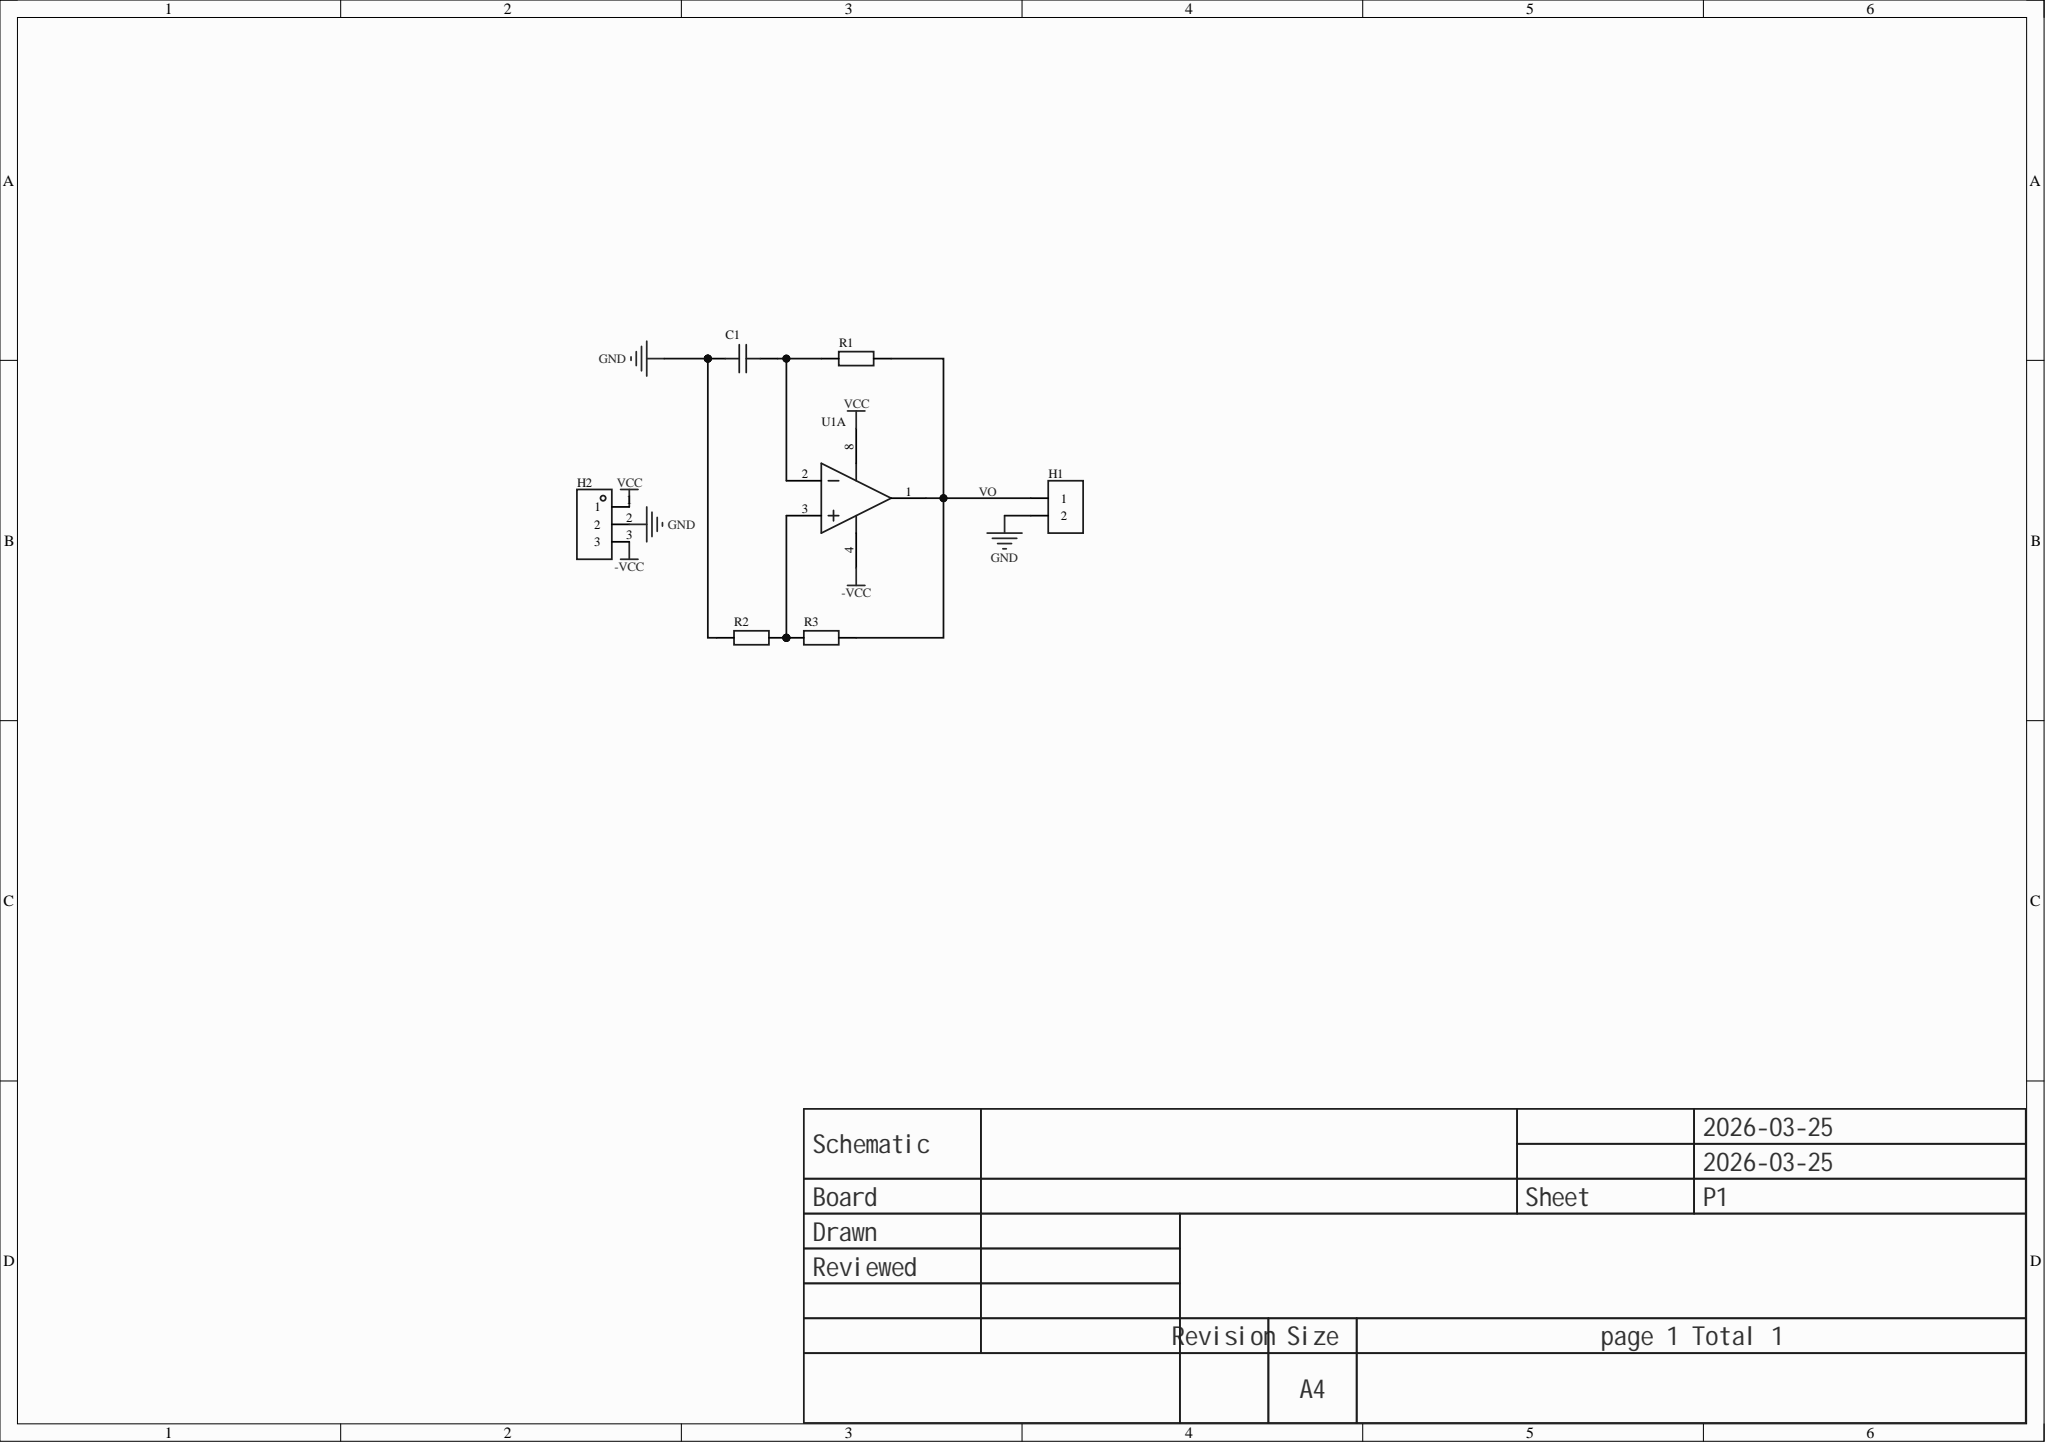Circuit board | Altium Designer | 7 parts | 6 nets
Bill of materials:
Comment,Description,Designator,Footprint,LibRef,Quantity
"100nF","","C1","C0603","CAP_0603","1"
"","","H1","HDR-TH_2P-P2.54-V-F","HDR-F_2.54_1x2P","1"
"","","H2","HDR-TH_3P-P2.54-V-M","HDR-M_2.54_1x3P","1"
"10K","","R1, R2, R3","R0603","Res_0603","3"
"NE5532DRG4","Amplifier type: -; Output power: -;","U1","SOIC-8_L5.0-W4.0-P1.27-LS6.0-BL","NE5532DRG4","1"
Netlist (Protel format):
[
C1
C0603
100nF



]
[
H1
HDR-TH_2P-P2.54-V-F




]
[
H2
HDR-TH_3P-P2.54-V-M




]
[
R1
R0603
10K



]
[
R2
R0603
10K



]
[
R3
R0603
10K



]
[
U1
SOIC-8_L5.0-W4.0-P1.27-LS6.0-BL
NE5532DRG4



]
(
VO
H1-1
R1-2
R3-2
U1-1
)
(
VCC
H2-1
U1-8
)
(
NetR2_2
R2-2
R3-1
U1-3
)
(
NetC1_2
C1-2
R1-1
U1-2
)
(
GND
C1-1
H1-2
H2-2
R2-1
)
(
-VCC
H2-3
U1-4
)